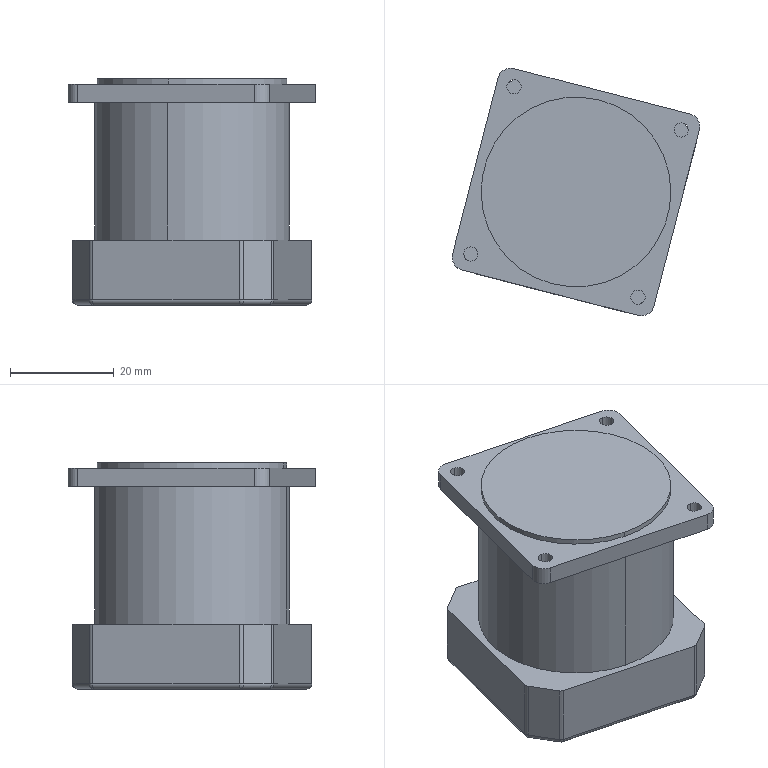Part | SolidWorks | features SplitBody 1 | 1 solid | 57 faces | box 47.65 x 47.65 x 43.5 mm | volume 55154 mm3 | cylinder 32 | plane 17 | sphere 8 | commonest cylinder face diameters 2 x16 2.75 x8 5 x4 36.5 x2 37.5 x2